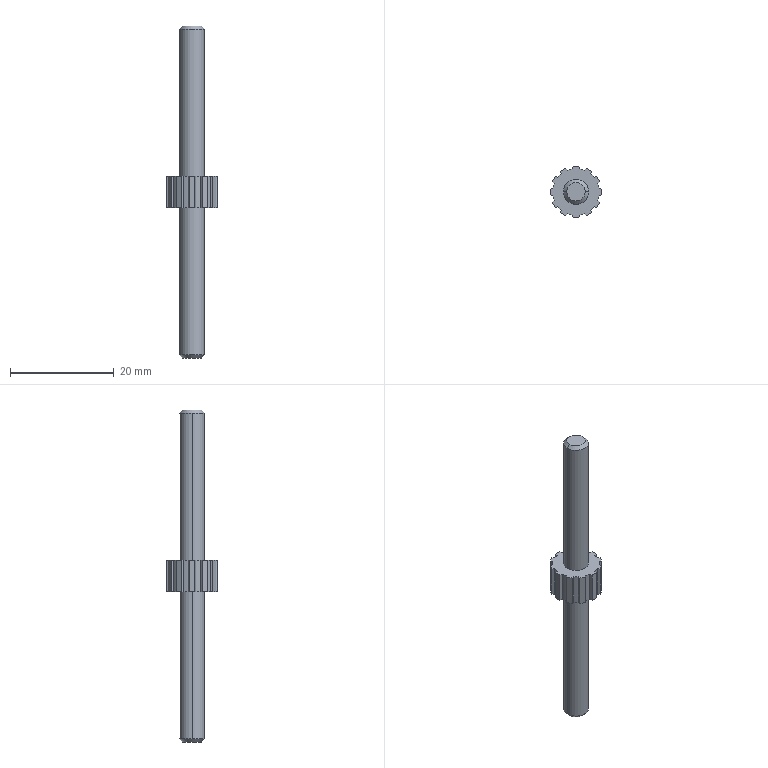Part | SolidWorks | features Extrusion 1, ICE 1, MirrorPattern 1, StudWizard 1 | 1 solid | 60 faces | box 9.896 x 9.896 x 64 mm | volume 1479 mm3 | plane 40 | cylinder 16 | cone 4 | commonest cylinder face diameters 9 x12 4.826 x4